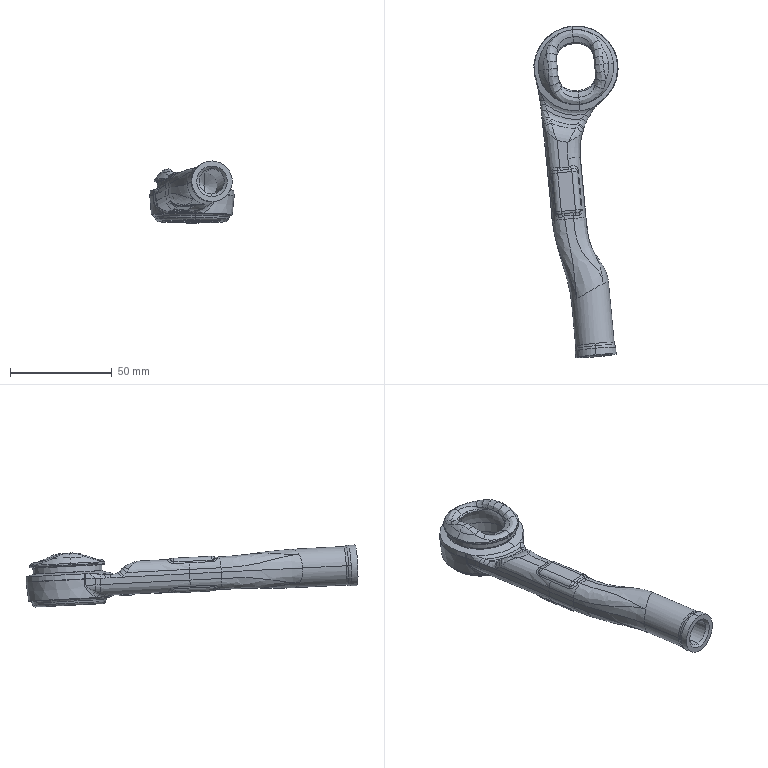Part | SolidWorks | features BaseBody 1 | 1 solid | 324 faces | box 41.492 x 163.305 x 30.52 mm | volume 40087 mm3 | spline 124 | plane 75 | torus 56 | cylinder 39 | cone 22 | sphere 8 | commonest cylinder face diameters 6 x16 12 x5 12.5 x2 19 x2 20 x2 27.76 x2